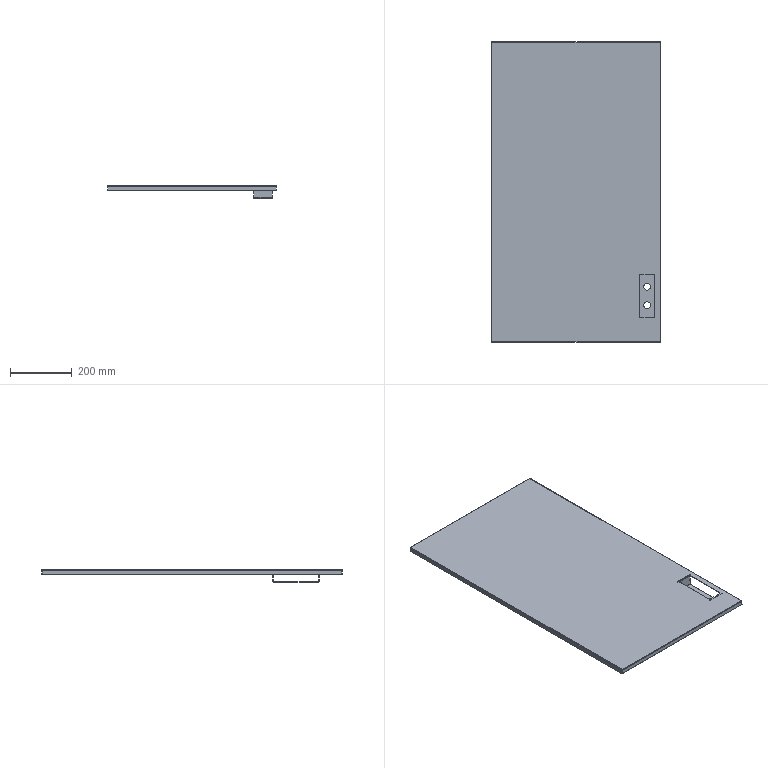Part | SolidWorks | features ICE 2, BossThin 1, FlatPattern 1, SMBaseFlange 1, SMMiteredFlange 1, SheetMetal 1 | 1 solid | 62 faces | box 550 x 973 x 40 mm | volume 869590 mm3 | plane 34 | cylinder 20 | spline 8 | commonest cylinder face diameters 1.473 x4 4.473 x4 10 x4 22 x4 3 x2 6 x2